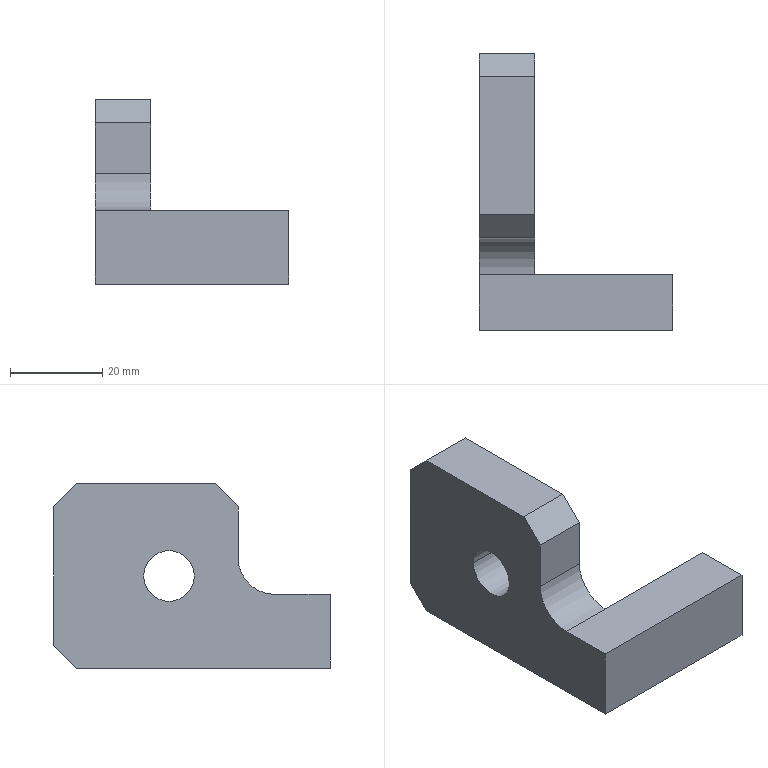Part | STEP file | 012-6-07-010 | 1 solid | 16 faces | box 42 x 60 x 40 mm | volume 27374 mm3 | plane 13 | cylinder 3 | commonest cylinder face diameters 11 x2 16 x1
STEP:
#1=CARTESIAN_POINT('',(0.,0.,0.));
#2=DIRECTION('',(0.,0.,1.));
#3=DIRECTION('',(1.,0.,0.));
#4=AXIS2_PLACEMENT_3D('',#1,#2,#3);
#5=CARTESIAN_POINT('',(0.,40.5,20.));
#6=VERTEX_POINT('',#5);
#7=CARTESIAN_POINT('',(12.,40.5,20.));
#8=VERTEX_POINT('',#7);
#9=CARTESIAN_POINT('',(-13.,40.5,20.));
#10=DIRECTION('',(1.,0.,0.));
#11=VECTOR('',#10,1.);
#12=LINE('',#9,#11);
#13=CARTESIAN_POINT('',(-13.,35.,20.));
#14=DIRECTION('',(1.,0.,0.));
#15=DIRECTION('',(0.,1.,0.));
#16=AXIS2_PLACEMENT_3D('',#13,#14,#15);
#17=CYLINDRICAL_SURFACE('',#16,5.5);
#18=CARTESIAN_POINT('',(6.283,0.));
#19=DIRECTION('',(0.,1.));
#20=VECTOR('',#19,1.);
#21=LINE('',#18,#20);
#22=(GEOMETRIC_REPRESENTATION_CONTEXT(2)PARAMETRIC_REPRESENTATION_CONTEXT()REPRESENTATION_CONTEXT('',''));
#23=DEFINITIONAL_REPRESENTATION('',(#21),#22);
#24=PCURVE('',#17,#23);
#25=CARTESIAN_POINT('',(-13.,35.,20.));
#26=DIRECTION('',(1.,0.,0.));
#27=DIRECTION('',(0.,1.,0.));
#28=AXIS2_PLACEMENT_3D('',#25,#26,#27);
#29=CYLINDRICAL_SURFACE('',#28,5.5);
#30=CARTESIAN_POINT('',(0.,0.));
#31=DIRECTION('',(0.,1.));
#32=VECTOR('',#31,1.);
#33=LINE('',#30,#32);
#34=(GEOMETRIC_REPRESENTATION_CONTEXT(2)PARAMETRIC_REPRESENTATION_CONTEXT()REPRESENTATION_CONTEXT('',''));
#35=DEFINITIONAL_REPRESENTATION('',(#33),#34);
#36=PCURVE('',#29,#35);
#37=SURFACE_CURVE('',#12,(#24,#36),.PCURVE_S1.);
#38=EDGE_CURVE('',#6,#8,#37,.T.);
#39=ORIENTED_EDGE('',*,*,#38,.T.);
#40=CARTESIAN_POINT('',(12.,29.5,20.));
#41=VERTEX_POINT('',#40);
#42=CARTESIAN_POINT('',(12.,35.,20.));
#43=DIRECTION('',(1.,0.,0.));
#44=DIRECTION('',(0.,1.,0.));
#45=AXIS2_PLACEMENT_3D('',#42,#43,#44);
#46=CIRCLE('',#45,5.5);
#47=CARTESIAN_POINT('',(0.,25.));
#48=DIRECTION('',(1.,0.));
#49=VECTOR('',#48,1.);
#50=LINE('',#47,#49);
#51=(GEOMETRIC_REPRESENTATION_CONTEXT(2)PARAMETRIC_REPRESENTATION_CONTEXT()REPRESENTATION_CONTEXT('',''));
#52=DEFINITIONAL_REPRESENTATION('',(#50),#51);
#53=PCURVE('',#17,#52);
#54=CARTESIAN_POINT('',(12.,60.,40.));
#55=DIRECTION('',(-1.,0.,0.));
#56=DIRECTION('',(0.,-1.,0.));
#57=AXIS2_PLACEMENT_3D('',#54,#55,#56);
#58=PLANE('',#57);
#59=CARTESIAN_POINT('',(19.5,-20.));
#60=CARTESIAN_POINT('',(19.5,-10.474));
#61=CARTESIAN_POINT('',(27.75,-15.237));
#62=CARTESIAN_POINT('',(36.,-20.));
#63=CARTESIAN_POINT('',(27.75,-24.763));
#64=CARTESIAN_POINT('',(19.5,-29.526));
#65=CARTESIAN_POINT('',(19.5,-20.));
#66=(BOUNDED_CURVE()B_SPLINE_CURVE(2,(#59,#60,#61,#62,#63,#64,#65),.UNSPECIFIED.,.T.,.F.)B_SPLINE_CURVE_WITH_KNOTS((1,2,2,2,2,1),(-2.094,0.,2.094,4.189,6.283,8.378),.UNSPECIFIED.)CURVE()GEOMETRIC_REPRESENTATION_ITEM()RATIONAL_B_SPLINE_CURVE((1.,0.5,1.,0.5,1.,0.5,1.))REPRESENTATION_ITEM(''));
#67=(GEOMETRIC_REPRESENTATION_CONTEXT(2)PARAMETRIC_REPRESENTATION_CONTEXT()REPRESENTATION_CONTEXT('',''));
#68=DEFINITIONAL_REPRESENTATION('',(#66),#67);
#69=PCURVE('',#58,#68);
#70=SURFACE_CURVE('',#46,(#53,#69),.PCURVE_S1.);
#71=EDGE_CURVE('',#41,#8,#70,.T.);
#72=ORIENTED_EDGE('',*,*,#71,.F.);
#73=CARTESIAN_POINT('',(0.,29.5,20.));
#74=VERTEX_POINT('',#73);
#75=CARTESIAN_POINT('',(-13.,29.5,20.));
#76=DIRECTION('',(1.,0.,0.));
#77=VECTOR('',#76,1.);
#78=LINE('',#75,#77);
#79=CARTESIAN_POINT('',(3.142,0.));
#80=DIRECTION('',(0.,1.));
#81=VECTOR('',#80,1.);
#82=LINE('',#79,#81);
#83=(GEOMETRIC_REPRESENTATION_CONTEXT(2)PARAMETRIC_REPRESENTATION_CONTEXT()REPRESENTATION_CONTEXT('',''));
#84=DEFINITIONAL_REPRESENTATION('',(#82),#83);
#85=PCURVE('',#17,#84);
#86=CARTESIAN_POINT('',(3.142,0.));
#87=DIRECTION('',(0.,1.));
#88=VECTOR('',#87,1.);
#89=LINE('',#86,#88);
#90=(GEOMETRIC_REPRESENTATION_CONTEXT(2)PARAMETRIC_REPRESENTATION_CONTEXT()REPRESENTATION_CONTEXT('',''));
#91=DEFINITIONAL_REPRESENTATION('',(#89),#90);
#92=PCURVE('',#29,#91);
#93=SURFACE_CURVE('',#78,(#85,#92),.PCURVE_S1.);
#94=EDGE_CURVE('',#74,#41,#93,.T.);
#95=ORIENTED_EDGE('',*,*,#94,.F.);
#96=CARTESIAN_POINT('',(0.,35.,20.));
#97=DIRECTION('',(1.,0.,0.));
#98=DIRECTION('',(0.,0.,-1.));
#99=AXIS2_PLACEMENT_3D('',#96,#97,#98);
#100=CIRCLE('',#99,5.5);
#101=CARTESIAN_POINT('',(-1.571,13.));
#102=DIRECTION('',(1.,0.));
#103=VECTOR('',#102,1.);
#104=LINE('',#101,#103);
#105=(GEOMETRIC_REPRESENTATION_CONTEXT(2)PARAMETRIC_REPRESENTATION_CONTEXT()REPRESENTATION_CONTEXT('',''));
#106=DEFINITIONAL_REPRESENTATION('',(#104),#105);
#107=PCURVE('',#17,#106);
#108=CARTESIAN_POINT('',(0.,0.,40.));
#109=DIRECTION('',(1.,0.,0.));
#110=DIRECTION('',(0.,0.,-1.));
#111=AXIS2_PLACEMENT_3D('',#108,#109,#110);
#112=PLANE('',#111);
#113=CARTESIAN_POINT('',(20.,35.));
#114=DIRECTION('',(1.,0.));
#115=AXIS2_PLACEMENT_2D('',#113,#114);
#116=CIRCLE('',#115,5.5);
#117=(GEOMETRIC_REPRESENTATION_CONTEXT(2)PARAMETRIC_REPRESENTATION_CONTEXT()REPRESENTATION_CONTEXT('',''));
#118=DEFINITIONAL_REPRESENTATION('',(#116),#117);
#119=PCURVE('',#112,#118);
#120=SURFACE_CURVE('',#100,(#107,#119),.PCURVE_S1.);
#121=EDGE_CURVE('',#74,#6,#120,.T.);
#122=ORIENTED_EDGE('',*,*,#121,.T.);
#123=EDGE_LOOP('',(#39,#72,#95,#122));
#124=FACE_BOUND('',#123,.F.);
#125=ADVANCED_FACE('',(#124),#17,.F.);
#126=CARTESIAN_POINT('',(0.,0.,16.));
#127=VERTEX_POINT('',#126);
#128=CARTESIAN_POINT('',(42.,0.,16.));
#129=VERTEX_POINT('',#128);
#130=CARTESIAN_POINT('',(42.,0.,16.));
#131=DIRECTION('',(1.,0.,0.));
#132=VECTOR('',#131,1.);
#133=LINE('',#130,#132);
#134=CARTESIAN_POINT('',(0.,0.,40.));
#135=DIRECTION('',(0.,1.,0.));
#136=DIRECTION('',(0.,0.,1.));
#137=AXIS2_PLACEMENT_3D('',#134,#135,#136);
#138=PLANE('',#137);
#139=CARTESIAN_POINT('',(-24.,42.));
#140=DIRECTION('',(0.,1.));
#141=VECTOR('',#140,1.);
#142=LINE('',#139,#141);
#143=(GEOMETRIC_REPRESENTATION_CONTEXT(2)PARAMETRIC_REPRESENTATION_CONTEXT()REPRESENTATION_CONTEXT('',''));
#144=DEFINITIONAL_REPRESENTATION('',(#142),#143);
#145=PCURVE('',#138,#144);
#146=CARTESIAN_POINT('',(42.,20.,16.));
#147=DIRECTION('',(0.,0.,1.));
#148=DIRECTION('',(1.,0.,0.));
#149=AXIS2_PLACEMENT_3D('',#146,#147,#148);
#150=PLANE('',#149);
#151=CARTESIAN_POINT('',(0.,-20.));
#152=DIRECTION('',(1.,0.));
#153=VECTOR('',#152,1.);
#154=LINE('',#151,#153);
#155=(GEOMETRIC_REPRESENTATION_CONTEXT(2)PARAMETRIC_REPRESENTATION_CONTEXT()REPRESENTATION_CONTEXT('',''));
#156=DEFINITIONAL_REPRESENTATION('',(#154),#155);
#157=PCURVE('',#150,#156);
#158=SURFACE_CURVE('',#133,(#145,#157),.PCURVE_S1.);
#159=EDGE_CURVE('',#127,#129,#158,.T.);
#160=ORIENTED_EDGE('',*,*,#159,.F.);
#161=CARTESIAN_POINT('',(0.,0.,0.));
#162=VERTEX_POINT('',#161);
#163=CARTESIAN_POINT('',(0.,0.,40.));
#164=DIRECTION('',(0.,0.,-1.));
#165=VECTOR('',#164,1.);
#166=LINE('',#163,#165);
#167=CARTESIAN_POINT('',(0.,0.));
#168=DIRECTION('',(-1.,0.));
#169=VECTOR('',#168,1.);
#170=LINE('',#167,#169);
#171=(GEOMETRIC_REPRESENTATION_CONTEXT(2)PARAMETRIC_REPRESENTATION_CONTEXT()REPRESENTATION_CONTEXT('',''));
#172=DEFINITIONAL_REPRESENTATION('',(#170),#171);
#173=PCURVE('',#138,#172);
#174=CARTESIAN_POINT('',(0.,0.));
#175=DIRECTION('',(1.,0.));
#176=VECTOR('',#175,1.);
#177=LINE('',#174,#176);
#178=(GEOMETRIC_REPRESENTATION_CONTEXT(2)PARAMETRIC_REPRESENTATION_CONTEXT()REPRESENTATION_CONTEXT('',''));
#179=DEFINITIONAL_REPRESENTATION('',(#177),#178);
#180=PCURVE('',#112,#179);
#181=SURFACE_CURVE('',#166,(#173,#180),.PCURVE_S1.);
#182=EDGE_CURVE('',#127,#162,#181,.T.);
#183=ORIENTED_EDGE('',*,*,#182,.T.);
#184=CARTESIAN_POINT('',(42.,0.,0.));
#185=VERTEX_POINT('',#184);
#186=CARTESIAN_POINT('',(0.,0.,0.));
#187=DIRECTION('',(1.,0.,0.));
#188=VECTOR('',#187,1.);
#189=LINE('',#186,#188);
#190=CARTESIAN_POINT('',(-40.,0.));
#191=DIRECTION('',(0.,1.));
#192=VECTOR('',#191,1.);
#193=LINE('',#190,#192);
#194=(GEOMETRIC_REPRESENTATION_CONTEXT(2)PARAMETRIC_REPRESENTATION_CONTEXT()REPRESENTATION_CONTEXT('',''));
#195=DEFINITIONAL_REPRESENTATION('',(#193),#194);
#196=PCURVE('',#138,#195);
#197=CARTESIAN_POINT('',(0.,60.,0.));
#198=DIRECTION('',(0.,0.,-1.));
#199=DIRECTION('',(-1.,0.,0.));
#200=AXIS2_PLACEMENT_3D('',#197,#198,#199);
#201=PLANE('',#200);
#202=CARTESIAN_POINT('',(0.,-60.));
#203=DIRECTION('',(-1.,0.));
#204=VECTOR('',#203,1.);
#205=LINE('',#202,#204);
#206=(GEOMETRIC_REPRESENTATION_CONTEXT(2)PARAMETRIC_REPRESENTATION_CONTEXT()REPRESENTATION_CONTEXT('',''));
#207=DEFINITIONAL_REPRESENTATION('',(#205),#206);
#208=PCURVE('',#201,#207);
#209=SURFACE_CURVE('',#189,(#196,#208),.PCURVE_S1.);
#210=EDGE_CURVE('',#162,#185,#209,.T.);
#211=ORIENTED_EDGE('',*,*,#210,.T.);
#212=CARTESIAN_POINT('',(42.,0.,40.));
#213=DIRECTION('',(0.,0.,-1.));
#214=VECTOR('',#213,1.);
#215=LINE('',#212,#214);
#216=CARTESIAN_POINT('',(0.,42.));
#217=DIRECTION('',(-1.,0.));
#218=VECTOR('',#217,1.);
#219=LINE('',#216,#218);
#220=(GEOMETRIC_REPRESENTATION_CONTEXT(2)PARAMETRIC_REPRESENTATION_CONTEXT()REPRESENTATION_CONTEXT('',''));
#221=DEFINITIONAL_REPRESENTATION('',(#219),#220);
#222=PCURVE('',#138,#221);
#223=CARTESIAN_POINT('',(42.,0.,40.));
#224=DIRECTION('',(-1.,0.,0.));
#225=DIRECTION('',(0.,0.,1.));
#226=AXIS2_PLACEMENT_3D('',#223,#224,#225);
#227=PLANE('',#226);
#228=CARTESIAN_POINT('',(0.,0.));
#229=DIRECTION('',(-1.,0.));
#230=VECTOR('',#229,1.);
#231=LINE('',#228,#230);
#232=(GEOMETRIC_REPRESENTATION_CONTEXT(2)PARAMETRIC_REPRESENTATION_CONTEXT()REPRESENTATION_CONTEXT('',''));
#233=DEFINITIONAL_REPRESENTATION('',(#231),#232);
#234=PCURVE('',#227,#233);
#235=SURFACE_CURVE('',#215,(#222,#234),.PCURVE_S1.);
#236=EDGE_CURVE('',#129,#185,#235,.T.);
#237=ORIENTED_EDGE('',*,*,#236,.F.);
#238=EDGE_LOOP('',(#160,#183,#211,#237));
#239=FACE_BOUND('',#238,.T.);
#240=ADVANCED_FACE('',(#239),#138,.F.);
#241=CARTESIAN_POINT('',(42.,12.,16.));
#242=VERTEX_POINT('',#241);
#243=CARTESIAN_POINT('',(42.,0.,16.));
#244=DIRECTION('',(0.,1.,0.));
#245=VECTOR('',#244,1.);
#246=LINE('',#243,#245);
#247=CARTESIAN_POINT('',(-24.,0.));
#248=DIRECTION('',(0.,1.));
#249=VECTOR('',#248,1.);
#250=LINE('',#247,#249);
#251=(GEOMETRIC_REPRESENTATION_CONTEXT(2)PARAMETRIC_REPRESENTATION_CONTEXT()REPRESENTATION_CONTEXT('',''));
#252=DEFINITIONAL_REPRESENTATION('',(#250),#251);
#253=PCURVE('',#227,#252);
#254=CARTESIAN_POINT('',(0.,-20.));
#255=DIRECTION('',(0.,1.));
#256=VECTOR('',#255,1.);
#257=LINE('',#254,#256);
#258=(GEOMETRIC_REPRESENTATION_CONTEXT(2)PARAMETRIC_REPRESENTATION_CONTEXT()REPRESENTATION_CONTEXT('',''));
#259=DEFINITIONAL_REPRESENTATION('',(#257),#258);
#260=PCURVE('',#150,#259);
#261=SURFACE_CURVE('',#246,(#253,#260),.PCURVE_S1.);
#262=EDGE_CURVE('',#129,#242,#261,.T.);
#263=ORIENTED_EDGE('',*,*,#262,.F.);
#264=ORIENTED_EDGE('',*,*,#236,.T.);
#265=CARTESIAN_POINT('',(42.,12.,0.));
#266=VERTEX_POINT('',#265);
#267=CARTESIAN_POINT('',(42.,0.,0.));
#268=DIRECTION('',(0.,1.,0.));
#269=VECTOR('',#268,1.);
#270=LINE('',#267,#269);
#271=CARTESIAN_POINT('',(-40.,0.));
#272=DIRECTION('',(0.,1.));
#273=VECTOR('',#272,1.);
#274=LINE('',#271,#273);
#275=(GEOMETRIC_REPRESENTATION_CONTEXT(2)PARAMETRIC_REPRESENTATION_CONTEXT()REPRESENTATION_CONTEXT('',''));
#276=DEFINITIONAL_REPRESENTATION('',(#274),#275);
#277=PCURVE('',#227,#276);
#278=CARTESIAN_POINT('',(-42.,-60.));
#279=DIRECTION('',(0.,1.));
#280=VECTOR('',#279,1.);
#281=LINE('',#278,#280);
#282=(GEOMETRIC_REPRESENTATION_CONTEXT(2)PARAMETRIC_REPRESENTATION_CONTEXT()REPRESENTATION_CONTEXT('',''));
#283=DEFINITIONAL_REPRESENTATION('',(#281),#282);
#284=PCURVE('',#201,#283);
#285=SURFACE_CURVE('',#270,(#277,#284),.PCURVE_S1.);
#286=EDGE_CURVE('',#185,#266,#285,.T.);
#287=ORIENTED_EDGE('',*,*,#286,.T.);
#288=CARTESIAN_POINT('',(42.,12.,40.));
#289=DIRECTION('',(0.,0.,-1.));
#290=VECTOR('',#289,1.);
#291=LINE('',#288,#290);
#292=CARTESIAN_POINT('',(0.,12.));
#293=DIRECTION('',(-1.,0.));
#294=VECTOR('',#293,1.);
#295=LINE('',#292,#294);
#296=(GEOMETRIC_REPRESENTATION_CONTEXT(2)PARAMETRIC_REPRESENTATION_CONTEXT()REPRESENTATION_CONTEXT('',''));
#297=DEFINITIONAL_REPRESENTATION('',(#295),#296);
#298=PCURVE('',#227,#297);
#299=CARTESIAN_POINT('',(12.,12.,40.));
#300=DIRECTION('',(0.,-1.,0.));
#301=DIRECTION('',(0.,0.,-1.));
#302=AXIS2_PLACEMENT_3D('',#299,#300,#301);
#303=PLANE('',#302);
#304=CARTESIAN_POINT('',(0.,30.));
#305=DIRECTION('',(1.,0.));
#306=VECTOR('',#305,1.);
#307=LINE('',#304,#306);
#308=(GEOMETRIC_REPRESENTATION_CONTEXT(2)PARAMETRIC_REPRESENTATION_CONTEXT()REPRESENTATION_CONTEXT('',''));
#309=DEFINITIONAL_REPRESENTATION('',(#307),#308);
#310=PCURVE('',#303,#309);
#311=SURFACE_CURVE('',#291,(#298,#310),.PCURVE_S1.);
#312=EDGE_CURVE('',#242,#266,#311,.T.);
#313=ORIENTED_EDGE('',*,*,#312,.F.);
#314=EDGE_LOOP('',(#263,#264,#287,#313));
#315=FACE_BOUND('',#314,.T.);
#316=ADVANCED_FACE('',(#315),#227,.F.);
#317=CARTESIAN_POINT('',(12.,12.,16.));
#318=VERTEX_POINT('',#317);
#319=CARTESIAN_POINT('',(12.,12.,16.));
#320=DIRECTION('',(-1.,0.,0.));
#321=VECTOR('',#320,1.);
#322=LINE('',#319,#321);
#323=CARTESIAN_POINT('',(24.,0.));
#324=DIRECTION('',(0.,-1.));
#325=VECTOR('',#324,1.);
#326=LINE('',#323,#325);
#327=(GEOMETRIC_REPRESENTATION_CONTEXT(2)PARAMETRIC_REPRESENTATION_CONTEXT()REPRESENTATION_CONTEXT('',''));
#328=DEFINITIONAL_REPRESENTATION('',(#326),#327);
#329=PCURVE('',#303,#328);
#330=CARTESIAN_POINT('',(-30.,-8.));
#331=DIRECTION('',(-1.,0.));
#332=VECTOR('',#331,1.);
#333=LINE('',#330,#332);
#334=(GEOMETRIC_REPRESENTATION_CONTEXT(2)PARAMETRIC_REPRESENTATION_CONTEXT()REPRESENTATION_CONTEXT('',''));
#335=DEFINITIONAL_REPRESENTATION('',(#333),#334);
#336=PCURVE('',#150,#335);
#337=SURFACE_CURVE('',#322,(#329,#336),.PCURVE_S1.);
#338=EDGE_CURVE('',#242,#318,#337,.T.);
#339=ORIENTED_EDGE('',*,*,#338,.F.);
#340=ORIENTED_EDGE('',*,*,#312,.T.);
#341=CARTESIAN_POINT('',(12.,12.,0.));
#342=VERTEX_POINT('',#341);
#343=CARTESIAN_POINT('',(12.,12.,0.));
#344=DIRECTION('',(-1.,0.,0.));
#345=VECTOR('',#344,1.);
#346=LINE('',#343,#345);
#347=CARTESIAN_POINT('',(40.,0.));
#348=DIRECTION('',(0.,-1.));
#349=VECTOR('',#348,1.);
#350=LINE('',#347,#349);
#351=(GEOMETRIC_REPRESENTATION_CONTEXT(2)PARAMETRIC_REPRESENTATION_CONTEXT()REPRESENTATION_CONTEXT('',''));
#352=DEFINITIONAL_REPRESENTATION('',(#350),#351);
#353=PCURVE('',#303,#352);
#354=CARTESIAN_POINT('',(-12.,-48.));
#355=DIRECTION('',(1.,0.));
#356=VECTOR('',#355,1.);
#357=LINE('',#354,#356);
#358=(GEOMETRIC_REPRESENTATION_CONTEXT(2)PARAMETRIC_REPRESENTATION_CONTEXT()REPRESENTATION_CONTEXT('',''));
#359=DEFINITIONAL_REPRESENTATION('',(#357),#358);
#360=PCURVE('',#201,#359);
#361=SURFACE_CURVE('',#346,(#353,#360),.PCURVE_S1.);
#362=EDGE_CURVE('',#266,#342,#361,.T.);
#363=ORIENTED_EDGE('',*,*,#362,.T.);
#364=CARTESIAN_POINT('',(12.,12.,40.));
#365=DIRECTION('',(0.,0.,-1.));
#366=VECTOR('',#365,1.);
#367=LINE('',#364,#366);
#368=CARTESIAN_POINT('',(0.,0.));
#369=DIRECTION('',(1.,0.));
#370=VECTOR('',#369,1.);
#371=LINE('',#368,#370);
#372=(GEOMETRIC_REPRESENTATION_CONTEXT(2)PARAMETRIC_REPRESENTATION_CONTEXT()REPRESENTATION_CONTEXT('',''));
#373=DEFINITIONAL_REPRESENTATION('',(#371),#372);
#374=PCURVE('',#303,#373);
#375=CARTESIAN_POINT('',(48.,0.));
#376=DIRECTION('',(0.,-1.));
#377=VECTOR('',#376,1.);
#378=LINE('',#375,#377);
#379=(GEOMETRIC_REPRESENTATION_CONTEXT(2)PARAMETRIC_REPRESENTATION_CONTEXT()REPRESENTATION_CONTEXT('',''));
#380=DEFINITIONAL_REPRESENTATION('',(#378),#379);
#381=PCURVE('',#58,#380);
#382=SURFACE_CURVE('',#367,(#374,#381),.PCURVE_S1.);
#383=EDGE_CURVE('',#318,#342,#382,.T.);
#384=ORIENTED_EDGE('',*,*,#383,.F.);
#385=EDGE_LOOP('',(#339,#340,#363,#384));
#386=FACE_BOUND('',#385,.T.);
#387=ADVANCED_FACE('',(#386),#303,.F.);
#388=CARTESIAN_POINT('',(0.,35.,20.));
#389=DIRECTION('',(1.,0.,0.));
#390=DIRECTION('',(0.,0.,-1.));
#391=AXIS2_PLACEMENT_3D('',#388,#389,#390);
#392=CIRCLE('',#391,5.5);
#393=CARTESIAN_POINT('',(20.,35.));
#394=DIRECTION('',(1.,0.));
#395=AXIS2_PLACEMENT_2D('',#393,#394);
#396=CIRCLE('',#395,5.5);
#397=(GEOMETRIC_REPRESENTATION_CONTEXT(2)PARAMETRIC_REPRESENTATION_CONTEXT()REPRESENTATION_CONTEXT('',''));
#398=DEFINITIONAL_REPRESENTATION('',(#396),#397);
#399=PCURVE('',#112,#398);
#400=CARTESIAN_POINT('',(-1.571,13.));
#401=DIRECTION('',(1.,0.));
#402=VECTOR('',#401,1.);
#403=LINE('',#400,#402);
#404=(GEOMETRIC_REPRESENTATION_CONTEXT(2)PARAMETRIC_REPRESENTATION_CONTEXT()REPRESENTATION_CONTEXT('',''));
#405=DEFINITIONAL_REPRESENTATION('',(#403),#404);
#406=PCURVE('',#29,#405);
#407=SURFACE_CURVE('',#392,(#399,#406),.PCURVE_S1.);
#408=EDGE_CURVE('',#6,#74,#407,.T.);
#409=ORIENTED_EDGE('',*,*,#408,.T.);
#410=ORIENTED_EDGE('',*,*,#121,.T.);
#411=EDGE_LOOP('',(#409,#410));
#412=FACE_BOUND('',#411,.T.);
#413=CARTESIAN_POINT('',(0.,20.,24.));
#414=VERTEX_POINT('',#413);
#415=CARTESIAN_POINT('',(0.,20.,35.));
#416=VERTEX_POINT('',#415);
#417=CARTESIAN_POINT('',(0.,20.,16.));
#418=DIRECTION('',(0.,0.,1.));
#419=VECTOR('',#418,1.);
#420=LINE('',#417,#419);
#421=CARTESIAN_POINT('',(24.,20.));
#422=DIRECTION('',(-1.,0.));
#423=VECTOR('',#422,1.);
#424=LINE('',#421,#423);
#425=(GEOMETRIC_REPRESENTATION_CONTEXT(2)PARAMETRIC_REPRESENTATION_CONTEXT()REPRESENTATION_CONTEXT('',''));
#426=DEFINITIONAL_REPRESENTATION('',(#424),#425);
#427=PCURVE('',#112,#426);
#428=CARTESIAN_POINT('',(42.,20.,16.));
#429=DIRECTION('',(0.,1.,0.));
#430=DIRECTION('',(-1.,0.,0.));
#431=AXIS2_PLACEMENT_3D('',#428,#429,#430);
#432=PLANE('',#431);
#433=CARTESIAN_POINT('',(42.,0.));
#434=DIRECTION('',(0.,1.));
#435=VECTOR('',#434,1.);
#436=LINE('',#433,#435);
#437=(GEOMETRIC_REPRESENTATION_CONTEXT(2)PARAMETRIC_REPRESENTATION_CONTEXT()REPRESENTATION_CONTEXT('',''));
#438=DEFINITIONAL_REPRESENTATION('',(#436),#437);
#439=PCURVE('',#432,#438);
#440=SURFACE_CURVE('',#420,(#427,#439),.PCURVE_S1.);
#441=EDGE_CURVE('',#414,#416,#440,.T.);
#442=ORIENTED_EDGE('',*,*,#441,.T.);
#443=CARTESIAN_POINT('',(0.,25.,40.));
#444=VERTEX_POINT('',#443);
#445=CARTESIAN_POINT('',(0.,25.,40.));
#446=DIRECTION('',(0.,0.7071,0.7071));
#447=VECTOR('',#446,1.);
#448=LINE('',#445,#447);
#449=CARTESIAN_POINT('',(0.,25.));
#450=DIRECTION('',(-0.7071,0.7071));
#451=VECTOR('',#450,1.);
#452=LINE('',#449,#451);
#453=(GEOMETRIC_REPRESENTATION_CONTEXT(2)PARAMETRIC_REPRESENTATION_CONTEXT()REPRESENTATION_CONTEXT('',''));
#454=DEFINITIONAL_REPRESENTATION('',(#452),#453);
#455=PCURVE('',#112,#454);
#456=CARTESIAN_POINT('',(0.,25.,40.));
#457=DIRECTION('',(0.,0.7071,-0.7071));
#458=DIRECTION('',(0.,0.7071,0.7071));
#459=AXIS2_PLACEMENT_3D('',#456,#457,#458);
#460=PLANE('',#459);
#461=CARTESIAN_POINT('',(0.,0.));
#462=DIRECTION('',(1.,0.));
#463=VECTOR('',#462,1.);
#464=LINE('',#461,#463);
#465=(GEOMETRIC_REPRESENTATION_CONTEXT(2)PARAMETRIC_REPRESENTATION_CONTEXT()REPRESENTATION_CONTEXT('',''));
#466=DEFINITIONAL_REPRESENTATION('',(#464),#465);
#467=PCURVE('',#460,#466);
#468=SURFACE_CURVE('',#448,(#455,#467),.PCURVE_S1.);
#469=EDGE_CURVE('',#416,#444,#468,.T.);
#470=ORIENTED_EDGE('',*,*,#469,.T.);
#471=CARTESIAN_POINT('',(0.,55.,40.));
#472=VERTEX_POINT('',#471);
#473=CARTESIAN_POINT('',(0.,0.,40.));
#474=DIRECTION('',(0.,-1.,0.));
#475=VECTOR('',#474,1.);
#476=LINE('',#473,#475);
#477=CARTESIAN_POINT('',(0.,0.));
#478=DIRECTION('',(0.,-1.));
#479=VECTOR('',#478,1.);
#480=LINE('',#477,#479);
#481=(GEOMETRIC_REPRESENTATION_CONTEXT(2)PARAMETRIC_REPRESENTATION_CONTEXT()REPRESENTATION_CONTEXT('',''));
#482=DEFINITIONAL_REPRESENTATION('',(#480),#481);
#483=PCURVE('',#112,#482);
#484=CARTESIAN_POINT('',(0.,60.,40.));
#485=DIRECTION('',(0.,0.,-1.));
#486=DIRECTION('',(-1.,0.,0.));
#487=AXIS2_PLACEMENT_3D('',#484,#485,#486);
#488=PLANE('',#487);
#489=CARTESIAN_POINT('',(0.,-60.));
#490=DIRECTION('',(0.,-1.));
#491=VECTOR('',#490,1.);
#492=LINE('',#489,#491);
#493=(GEOMETRIC_REPRESENTATION_CONTEXT(2)PARAMETRIC_REPRESENTATION_CONTEXT()REPRESENTATION_CONTEXT('',''));
#494=DEFINITIONAL_REPRESENTATION('',(#492),#493);
#495=PCURVE('',#488,#494);
#496=SURFACE_CURVE('',#476,(#483,#495),.PCURVE_S1.);
#497=EDGE_CURVE('',#472,#444,#496,.T.);
#498=ORIENTED_EDGE('',*,*,#497,.F.);
#499=CARTESIAN_POINT('',(0.,60.,35.));
#500=VERTEX_POINT('',#499);
#501=CARTESIAN_POINT('',(0.,55.,40.));
#502=DIRECTION('',(0.,0.7071,-0.7071));
#503=VECTOR('',#502,1.);
#504=LINE('',#501,#503);
#505=CARTESIAN_POINT('',(0.,55.));
#506=DIRECTION('',(0.7071,0.7071));
#507=VECTOR('',#506,1.);
#508=LINE('',#505,#507);
#509=(GEOMETRIC_REPRESENTATION_CONTEXT(2)PARAMETRIC_REPRESENTATION_CONTEXT()REPRESENTATION_CONTEXT('',''));
#510=DEFINITIONAL_REPRESENTATION('',(#508),#509);
#511=PCURVE('',#112,#510);
#512=CARTESIAN_POINT('',(0.,55.,40.));
#513=DIRECTION('',(0.,-0.7071,-0.7071));
#514=DIRECTION('',(0.,0.7071,-0.7071));
#515=AXIS2_PLACEMENT_3D('',#512,#513,#514);
#516=PLANE('',#515);
#517=CARTESIAN_POINT('',(0.,0.));
#518=DIRECTION('',(1.,0.));
#519=VECTOR('',#518,1.);
#520=LINE('',#517,#519);
#521=(GEOMETRIC_REPRESENTATION_CONTEXT(2)PARAMETRIC_REPRESENTATION_CONTEXT()REPRESENTATION_CONTEXT('',''));
#522=DEFINITIONAL_REPRESENTATION('',(#520),#521);
#523=PCURVE('',#516,#522);
#524=SURFACE_CURVE('',#504,(#511,#523),.PCURVE_S1.);
#525=EDGE_CURVE('',#472,#500,#524,.T.);
#526=ORIENTED_EDGE('',*,*,#525,.T.);
#527=CARTESIAN_POINT('',(0.,60.,5.));
#528=VERTEX_POINT('',#527);
#529=CARTESIAN_POINT('',(0.,60.,40.));
#530=DIRECTION('',(0.,0.,-1.));
#531=VECTOR('',#530,1.);
#532=LINE('',#529,#531);
#533=CARTESIAN_POINT('',(0.,60.));
#534=DIRECTION('',(1.,0.));
#535=VECTOR('',#534,1.);
#536=LINE('',#533,#535);
#537=(GEOMETRIC_REPRESENTATION_CONTEXT(2)PARAMETRIC_REPRESENTATION_CONTEXT()REPRESENTATION_CONTEXT('',''));
#538=DEFINITIONAL_REPRESENTATION('',(#536),#537);
#539=PCURVE('',#112,#538);
#540=CARTESIAN_POINT('',(0.,60.,40.));
#541=DIRECTION('',(0.,-1.,0.));
#542=DIRECTION('',(0.,0.,-1.));
#543=AXIS2_PLACEMENT_3D('',#540,#541,#542);
#544=PLANE('',#543);
#545=CARTESIAN_POINT('',(0.,0.));
#546=DIRECTION('',(1.,0.));
#547=VECTOR('',#546,1.);
#548=LINE('',#545,#547);
#549=(GEOMETRIC_REPRESENTATION_CONTEXT(2)PARAMETRIC_REPRESENTATION_CONTEXT()REPRESENTATION_CONTEXT('',''));
#550=DEFINITIONAL_REPRESENTATION('',(#548),#549);
#551=PCURVE('',#544,#550);
#552=SURFACE_CURVE('',#532,(#539,#551),.PCURVE_S1.);
#553=EDGE_CURVE('',#500,#528,#552,.T.);
#554=ORIENTED_EDGE('',*,*,#553,.T.);
#555=CARTESIAN_POINT('',(0.,55.,0.));
#556=VERTEX_POINT('',#555);
#557=CARTESIAN_POINT('',(0.,60.,5.));
#558=DIRECTION('',(0.,-0.7071,-0.7071));
#559=VECTOR('',#558,1.);
#560=LINE('',#557,#559);
#561=CARTESIAN_POINT('',(35.,60.));
#562=DIRECTION('',(0.7071,-0.7071));
#563=VECTOR('',#562,1.);
#564=LINE('',#561,#563);
#565=(GEOMETRIC_REPRESENTATION_CONTEXT(2)PARAMETRIC_REPRESENTATION_CONTEXT()REPRESENTATION_CONTEXT('',''));
#566=DEFINITIONAL_REPRESENTATION('',(#564),#565);
#567=PCURVE('',#112,#566);
#568=CARTESIAN_POINT('',(0.,60.,5.));
#569=DIRECTION('',(0.,0.7071,-0.7071));
#570=DIRECTION('',(0.,0.7071,0.7071));
#571=AXIS2_PLACEMENT_3D('',#568,#569,#570);
#572=PLANE('',#571);
#573=CARTESIAN_POINT('',(0.,0.));
#574=DIRECTION('',(-1.,0.));
#575=VECTOR('',#574,1.);
#576=LINE('',#573,#575);
#577=(GEOMETRIC_REPRESENTATION_CONTEXT(2)PARAMETRIC_REPRESENTATION_CONTEXT()REPRESENTATION_CONTEXT('',''));
#578=DEFINITIONAL_REPRESENTATION('',(#576),#577);
#579=PCURVE('',#572,#578);
#580=SURFACE_CURVE('',#560,(#567,#579),.PCURVE_S1.);
#581=EDGE_CURVE('',#528,#556,#580,.T.);
#582=ORIENTED_EDGE('',*,*,#581,.T.);
#583=CARTESIAN_POINT('',(0.,0.,0.));
#584=DIRECTION('',(0.,-1.,0.));
#585=VECTOR('',#584,1.);
#586=LINE('',#583,#585);
#587=CARTESIAN_POINT('',(40.,0.));
#588=DIRECTION('',(0.,-1.));
#589=VECTOR('',#588,1.);
#590=LINE('',#587,#589);
#591=(GEOMETRIC_REPRESENTATION_CONTEXT(2)PARAMETRIC_REPRESENTATION_CONTEXT()REPRESENTATION_CONTEXT('',''));
#592=DEFINITIONAL_REPRESENTATION('',(#590),#591);
#593=PCURVE('',#112,#592);
#594=CARTESIAN_POINT('',(0.,-60.));
#595=DIRECTION('',(0.,-1.));
#596=VECTOR('',#595,1.);
#597=LINE('',#594,#596);
#598=(GEOMETRIC_REPRESENTATION_CONTEXT(2)PARAMETRIC_REPRESENTATION_CONTEXT()REPRESENTATION_CONTEXT('',''));
#599=DEFINITIONAL_REPRESENTATION('',(#597),#598);
#600=PCURVE('',#201,#599);
#601=SURFACE_CURVE('',#586,(#593,#600),.PCURVE_S1.);
#602=EDGE_CURVE('',#556,#162,#601,.T.);
#603=ORIENTED_EDGE('',*,*,#602,.T.);
#604=ORIENTED_EDGE('',*,*,#182,.F.);
#605=CARTESIAN_POINT('',(0.,12.,16.));
#606=VERTEX_POINT('',#605);
#607=CARTESIAN_POINT('',(0.,0.,16.));
#608=DIRECTION('',(0.,-1.,0.));
#609=VECTOR('',#608,1.);
#610=LINE('',#607,#609);
#611=CARTESIAN_POINT('',(24.,0.));
#612=DIRECTION('',(0.,-1.));
#613=VECTOR('',#612,1.);
#614=LINE('',#611,#613);
#615=(GEOMETRIC_REPRESENTATION_CONTEXT(2)PARAMETRIC_REPRESENTATION_CONTEXT()REPRESENTATION_CONTEXT('',''));
#616=DEFINITIONAL_REPRESENTATION('',(#614),#615);
#617=PCURVE('',#112,#616);
#618=CARTESIAN_POINT('',(-42.,-20.));
#619=DIRECTION('',(0.,-1.));
#620=VECTOR('',#619,1.);
#621=LINE('',#618,#620);
#622=(GEOMETRIC_REPRESENTATION_CONTEXT(2)PARAMETRIC_REPRESENTATION_CONTEXT()REPRESENTATION_CONTEXT('',''));
#623=DEFINITIONAL_REPRESENTATION('',(#621),#622);
#624=PCURVE('',#150,#623);
#625=SURFACE_CURVE('',#610,(#617,#624),.PCURVE_S1.);
#626=EDGE_CURVE('',#606,#127,#625,.T.);
#627=ORIENTED_EDGE('',*,*,#626,.F.);
#628=CARTESIAN_POINT('',(0.,12.,24.));
#629=DIRECTION('',(1.,0.,0.));
#630=DIRECTION('',(0.,0.,-1.));
#631=AXIS2_PLACEMENT_3D('',#628,#629,#630);
#632=CIRCLE('',#631,8.);
#633=CARTESIAN_POINT('',(16.,12.));
#634=DIRECTION('',(1.,0.));
#635=AXIS2_PLACEMENT_2D('',#633,#634);
#636=CIRCLE('',#635,8.);
#637=(GEOMETRIC_REPRESENTATION_CONTEXT(2)PARAMETRIC_REPRESENTATION_CONTEXT()REPRESENTATION_CONTEXT('',''));
#638=DEFINITIONAL_REPRESENTATION('',(#636),#637);
#639=PCURVE('',#112,#638);
#640=CARTESIAN_POINT('',(42.,12.,24.));
#641=DIRECTION('',(-1.,0.,0.));
#642=DIRECTION('',(0.,-1.,0.));
#643=AXIS2_PLACEMENT_3D('',#640,#641,#642);
#644=CYLINDRICAL_SURFACE('',#643,8.);
#645=CARTESIAN_POINT('',(4.712,42.));
#646=DIRECTION('',(-1.,0.));
#647=VECTOR('',#646,1.);
#648=LINE('',#645,#647);
#649=(GEOMETRIC_REPRESENTATION_CONTEXT(2)PARAMETRIC_REPRESENTATION_CONTEXT()REPRESENTATION_CONTEXT('',''));
#650=DEFINITIONAL_REPRESENTATION('',(#648),#649);
#651=PCURVE('',#644,#650);
#652=SURFACE_CURVE('',#632,(#639,#651),.PCURVE_S1.);
#653=EDGE_CURVE('',#606,#414,#652,.T.);
#654=ORIENTED_EDGE('',*,*,#653,.T.);
#655=EDGE_LOOP('',(#442,#470,#498,#526,#554,#582,#603,#604,#627,#654));
#656=FACE_BOUND('',#655,.T.);
#657=ADVANCED_FACE('',(#412,#656),#112,.F.);
#658=CARTESIAN_POINT('',(12.,35.,20.));
#659=DIRECTION('',(1.,0.,0.));
#660=DIRECTION('',(0.,1.,0.));
#661=AXIS2_PLACEMENT_3D('',#658,#659,#660);
#662=CIRCLE('',#661,5.5);
#663=CARTESIAN_POINT('',(19.5,-20.));
#664=CARTESIAN_POINT('',(19.5,-10.474));
#665=CARTESIAN_POINT('',(27.75,-15.237));
#666=CARTESIAN_POINT('',(36.,-20.));
#667=CARTESIAN_POINT('',(27.75,-24.763));
#668=CARTESIAN_POINT('',(19.5,-29.526));
#669=CARTESIAN_POINT('',(19.5,-20.));
#670=(BOUNDED_CURVE()B_SPLINE_CURVE(2,(#663,#664,#665,#666,#667,#668,#669),.UNSPECIFIED.,.T.,.F.)B_SPLINE_CURVE_WITH_KNOTS((1,2,2,2,2,1),(-2.094,0.,2.094,4.189,6.283,8.378),.UNSPECIFIED.)CURVE()GEOMETRIC_REPRESENTATION_ITEM()RATIONAL_B_SPLINE_CURVE((1.,0.5,1.,0.5,1.,0.5,1.))REPRESENTATION_ITEM(''));
#671=(GEOMETRIC_REPRESENTATION_CONTEXT(2)PARAMETRIC_REPRESENTATION_CONTEXT()REPRESENTATION_CONTEXT('',''));
#672=DEFINITIONAL_REPRESENTATION('',(#670),#671);
#673=PCURVE('',#58,#672);
#674=CARTESIAN_POINT('',(0.,25.));
#675=DIRECTION('',(1.,0.));
#676=VECTOR('',#675,1.);
#677=LINE('',#674,#676);
#678=(GEOMETRIC_REPRESENTATION_CONTEXT(2)PARAMETRIC_REPRESENTATION_CONTEXT()REPRESENTATION_CONTEXT('',''));
#679=DEFINITIONAL_REPRESENTATION('',(#677),#678);
#680=PCURVE('',#29,#679);
#681=SURFACE_CURVE('',#662,(#673,#680),.PCURVE_S1.);
#682=EDGE_CURVE('',#8,#41,#681,.T.);
#683=ORIENTED_EDGE('',*,*,#682,.F.);
#684=ORIENTED_EDGE('',*,*,#71,.F.);
#685=EDGE_LOOP('',(#683,#684));
#686=FACE_BOUND('',#685,.T.);
#687=CARTESIAN_POINT('',(12.,25.,40.));
#688=VERTEX_POINT('',#687);
#689=CARTESIAN_POINT('',(12.,55.,40.));
#690=VERTEX_POINT('',#689);
#691=CARTESIAN_POINT('',(12.,60.,40.));
#692=DIRECTION('',(0.,1.,0.));
#693=VECTOR('',#692,1.);
#694=LINE('',#691,#693);
#695=CARTESIAN_POINT('',(0.,0.));
#696=DIRECTION('',(-1.,0.));
#697=VECTOR('',#696,1.);
#698=LINE('',#695,#697);
#699=(GEOMETRIC_REPRESENTATION_CONTEXT(2)PARAMETRIC_REPRESENTATION_CONTEXT()REPRESENTATION_CONTEXT('',''));
#700=DEFINITIONAL_REPRESENTATION('',(#698),#699);
#701=PCURVE('',#58,#700);
#702=CARTESIAN_POINT('',(-12.,0.));
#703=DIRECTION('',(0.,1.));
#704=VECTOR('',#703,1.);
#705=LINE('',#702,#704);
#706=(GEOMETRIC_REPRESENTATION_CONTEXT(2)PARAMETRIC_REPRESENTATION_CONTEXT()REPRESENTATION_CONTEXT('',''));
#707=DEFINITIONAL_REPRESENTATION('',(#705),#706);
#708=PCURVE('',#488,#707);
#709=SURFACE_CURVE('',#694,(#701,#708),.PCURVE_S1.);
#710=EDGE_CURVE('',#688,#690,#709,.T.);
#711=ORIENTED_EDGE('',*,*,#710,.F.);
#712=CARTESIAN_POINT('',(12.,20.,35.));
#713=VERTEX_POINT('',#712);
#714=CARTESIAN_POINT('',(12.,25.,40.));
#715=DIRECTION('',(0.,-0.7071,-0.7071));
#716=VECTOR('',#715,1.);
#717=LINE('',#714,#716);
#718=CARTESIAN_POINT('',(35.,0.));
#719=DIRECTION('',(0.7071,-0.7071));
#720=VECTOR('',#719,1.);
#721=LINE('',#718,#720);
#722=(GEOMETRIC_REPRESENTATION_CONTEXT(2)PARAMETRIC_REPRESENTATION_CONTEXT()REPRESENTATION_CONTEXT('',''));
#723=DEFINITIONAL_REPRESENTATION('',(#721),#722);
#724=PCURVE('',#58,#723);
#725=CARTESIAN_POINT('',(0.,12.));
#726=DIRECTION('',(-1.,0.));
#727=VECTOR('',#726,1.);
#728=LINE('',#725,#727);
#729=(GEOMETRIC_REPRESENTATION_CONTEXT(2)PARAMETRIC_REPRESENTATION_CONTEXT()REPRESENTATION_CONTEXT('',''));
#730=DEFINITIONAL_REPRESENTATION('',(#728),#729);
#731=PCURVE('',#460,#730);
#732=SURFACE_CURVE('',#717,(#724,#731),.PCURVE_S1.);
#733=EDGE_CURVE('',#688,#713,#732,.T.);
#734=ORIENTED_EDGE('',*,*,#733,.T.);
#735=CARTESIAN_POINT('',(12.,20.,24.));
#736=VERTEX_POINT('',#735);
#737=CARTESIAN_POINT('',(12.,20.,40.));
#738=DIRECTION('',(0.,0.,-1.));
#739=VECTOR('',#738,1.);
#740=LINE('',#737,#739);
#741=CARTESIAN_POINT('',(40.,0.));
#742=DIRECTION('',(0.,-1.));
#743=VECTOR('',#742,1.);
#744=LINE('',#741,#743);
#745=(GEOMETRIC_REPRESENTATION_CONTEXT(2)PARAMETRIC_REPRESENTATION_CONTEXT()REPRESENTATION_CONTEXT('',''));
#746=DEFINITIONAL_REPRESENTATION('',(#744),#745);
#747=PCURVE('',#58,#746);
#748=CARTESIAN_POINT('',(30.,24.));
#749=DIRECTION('',(0.,-1.));
#750=VECTOR('',#749,1.);
#751=LINE('',#748,#750);
#752=(GEOMETRIC_REPRESENTATION_CONTEXT(2)PARAMETRIC_REPRESENTATION_CONTEXT()REPRESENTATION_CONTEXT('',''));
#753=DEFINITIONAL_REPRESENTATION('',(#751),#752);
#754=PCURVE('',#432,#753);
#755=SURFACE_CURVE('',#740,(#747,#754),.PCURVE_S1.);
#756=EDGE_CURVE('',#713,#736,#755,.T.);
#757=ORIENTED_EDGE('',*,*,#756,.T.);
#758=CARTESIAN_POINT('',(12.,12.,24.));
#759=DIRECTION('',(-1.,0.,0.));
#760=DIRECTION('',(0.,-1.,0.));
#761=AXIS2_PLACEMENT_3D('',#758,#759,#760);
#762=CIRCLE('',#761,8.);
#763=CARTESIAN_POINT('',(48.,-16.));
#764=DIRECTION('',(1.,0.));
#765=AXIS2_PLACEMENT_2D('',#763,#764);
#766=CIRCLE('',#765,8.);
#767=(GEOMETRIC_REPRESENTATION_CONTEXT(2)PARAMETRIC_REPRESENTATION_CONTEXT()REPRESENTATION_CONTEXT('',''));
#768=DEFINITIONAL_REPRESENTATION('',(#766),#767);
#769=PCURVE('',#58,#768);
#770=CARTESIAN_POINT('',(0.,30.));
#771=DIRECTION('',(1.,0.));
#772=VECTOR('',#771,1.);
#773=LINE('',#770,#772);
#774=(GEOMETRIC_REPRESENTATION_CONTEXT(2)PARAMETRIC_REPRESENTATION_CONTEXT()REPRESENTATION_CONTEXT('',''));
#775=DEFINITIONAL_REPRESENTATION('',(#773),#774);
#776=PCURVE('',#644,#775);
#777=SURFACE_CURVE('',#762,(#769,#776),.PCURVE_S1.);
#778=EDGE_CURVE('',#736,#318,#777,.T.);
#779=ORIENTED_EDGE('',*,*,#778,.T.);
#780=ORIENTED_EDGE('',*,*,#383,.T.);
#781=CARTESIAN_POINT('',(12.,55.,0.));
#782=VERTEX_POINT('',#781);
#783=CARTESIAN_POINT('',(12.,60.,0.));
#784=DIRECTION('',(0.,1.,0.));
#785=VECTOR('',#784,1.);
#786=LINE('',#783,#785);
#787=CARTESIAN_POINT('',(0.,-40.));
#788=DIRECTION('',(-1.,0.));
#789=VECTOR('',#788,1.);
#790=LINE('',#787,#789);
#791=(GEOMETRIC_REPRESENTATION_CONTEXT(2)PARAMETRIC_REPRESENTATION_CONTEXT()REPRESENTATION_CONTEXT('',''));
#792=DEFINITIONAL_REPRESENTATION('',(#790),#791);
#793=PCURVE('',#58,#792);
#794=CARTESIAN_POINT('',(-12.,0.));
#795=DIRECTION('',(0.,1.));
#796=VECTOR('',#795,1.);
#797=LINE('',#794,#796);
#798=(GEOMETRIC_REPRESENTATION_CONTEXT(2)PARAMETRIC_REPRESENTATION_CONTEXT()REPRESENTATION_CONTEXT('',''));
#799=DEFINITIONAL_REPRESENTATION('',(#797),#798);
#800=PCURVE('',#201,#799);
#801=SURFACE_CURVE('',#786,(#793,#800),.PCURVE_S1.);
#802=EDGE_CURVE('',#342,#782,#801,.T.);
#803=ORIENTED_EDGE('',*,*,#802,.T.);
#804=CARTESIAN_POINT('',(12.,60.,5.));
#805=VERTEX_POINT('',#804);
#806=CARTESIAN_POINT('',(12.,60.,5.));
#807=DIRECTION('',(0.,0.7071,0.7071));
#808=VECTOR('',#807,1.);
#809=LINE('',#806,#808);
#810=CARTESIAN_POINT('',(0.,-35.));
#811=DIRECTION('',(-0.7071,0.7071));
#812=VECTOR('',#811,1.);
#813=LINE('',#810,#812);
#814=(GEOMETRIC_REPRESENTATION_CONTEXT(2)PARAMETRIC_REPRESENTATION_CONTEXT()REPRESENTATION_CONTEXT('',''));
#815=DEFINITIONAL_REPRESENTATION('',(#813),#814);
#816=PCURVE('',#58,#815);
#817=CARTESIAN_POINT('',(0.,12.));
#818=DIRECTION('',(1.,0.));
#819=VECTOR('',#818,1.);
#820=LINE('',#817,#819);
#821=(GEOMETRIC_REPRESENTATION_CONTEXT(2)PARAMETRIC_REPRESENTATION_CONTEXT()REPRESENTATION_CONTEXT('',''));
#822=DEFINITIONAL_REPRESENTATION('',(#820),#821);
#823=PCURVE('',#572,#822);
#824=SURFACE_CURVE('',#809,(#816,#823),.PCURVE_S1.);
#825=EDGE_CURVE('',#782,#805,#824,.T.);
#826=ORIENTED_EDGE('',*,*,#825,.T.);
#827=CARTESIAN_POINT('',(12.,60.,35.));
#828=VERTEX_POINT('',#827);
#829=CARTESIAN_POINT('',(12.,60.,40.));
#830=DIRECTION('',(0.,0.,-1.));
#831=VECTOR('',#830,1.);
#832=LINE('',#829,#831);
#833=CARTESIAN_POINT('',(0.,0.));
#834=DIRECTION('',(0.,-1.));
#835=VECTOR('',#834,1.);
#836=LINE('',#833,#835);
#837=(GEOMETRIC_REPRESENTATION_CONTEXT(2)PARAMETRIC_REPRESENTATION_CONTEXT()REPRESENTATION_CONTEXT('',''));
#838=DEFINITIONAL_REPRESENTATION('',(#836),#837);
#839=PCURVE('',#58,#838);
#840=CARTESIAN_POINT('',(0.,12.));
#841=DIRECTION('',(1.,0.));
#842=VECTOR('',#841,1.);
#843=LINE('',#840,#842);
#844=(GEOMETRIC_REPRESENTATION_CONTEXT(2)PARAMETRIC_REPRESENTATION_CONTEXT()REPRESENTATION_CONTEXT('',''));
#845=DEFINITIONAL_REPRESENTATION('',(#843),#844);
#846=PCURVE('',#544,#845);
#847=SURFACE_CURVE('',#832,(#839,#846),.PCURVE_S1.);
#848=EDGE_CURVE('',#828,#805,#847,.T.);
#849=ORIENTED_EDGE('',*,*,#848,.F.);
#850=CARTESIAN_POINT('',(12.,55.,40.));
#851=DIRECTION('',(0.,-0.7071,0.7071));
#852=VECTOR('',#851,1.);
#853=LINE('',#850,#852);
#854=CARTESIAN_POINT('',(5.,0.));
#855=DIRECTION('',(0.7071,0.7071));
#856=VECTOR('',#855,1.);
#857=LINE('',#854,#856);
#858=(GEOMETRIC_REPRESENTATION_CONTEXT(2)PARAMETRIC_REPRESENTATION_CONTEXT()REPRESENTATION_CONTEXT('',''));
#859=DEFINITIONAL_REPRESENTATION('',(#857),#858);
#860=PCURVE('',#58,#859);
#861=CARTESIAN_POINT('',(0.,12.));
#862=DIRECTION('',(-1.,0.));
#863=VECTOR('',#862,1.);
#864=LINE('',#861,#863);
#865=(GEOMETRIC_REPRESENTATION_CONTEXT(2)PARAMETRIC_REPRESENTATION_CONTEXT()REPRESENTATION_CONTEXT('',''));
#866=DEFINITIONAL_REPRESENTATION('',(#864),#865);
#867=PCURVE('',#516,#866);
#868=SURFACE_CURVE('',#853,(#860,#867),.PCURVE_S1.);
#869=EDGE_CURVE('',#828,#690,#868,.T.);
#870=ORIENTED_EDGE('',*,*,#869,.T.);
#871=EDGE_LOOP('',(#711,#734,#757,#779,#780,#803,#826,#849,#870));
#872=FACE_BOUND('',#871,.T.);
#873=ADVANCED_FACE('',(#686,#872),#58,.F.);
#874=ORIENTED_EDGE('',*,*,#848,.T.);
#875=CARTESIAN_POINT('',(0.,60.,5.));
#876=DIRECTION('',(-1.,0.,0.));
#877=VECTOR('',#876,1.);
#878=LINE('',#875,#877);
#879=CARTESIAN_POINT('',(35.,0.));
#880=DIRECTION('',(0.,-1.));
#881=VECTOR('',#880,1.);
#882=LINE('',#879,#881);
#883=(GEOMETRIC_REPRESENTATION_CONTEXT(2)PARAMETRIC_REPRESENTATION_CONTEXT()REPRESENTATION_CONTEXT('',''));
#884=DEFINITIONAL_REPRESENTATION('',(#882),#883);
#885=PCURVE('',#544,#884);
#886=CARTESIAN_POINT('',(0.,0.));
#887=DIRECTION('',(0.,-1.));
#888=VECTOR('',#887,1.);
#889=LINE('',#886,#888);
#890=(GEOMETRIC_REPRESENTATION_CONTEXT(2)PARAMETRIC_REPRESENTATION_CONTEXT()REPRESENTATION_CONTEXT('',''));
#891=DEFINITIONAL_REPRESENTATION('',(#889),#890);
#892=PCURVE('',#572,#891);
#893=SURFACE_CURVE('',#878,(#885,#892),.PCURVE_S1.);
#894=EDGE_CURVE('',#805,#528,#893,.T.);
#895=ORIENTED_EDGE('',*,*,#894,.T.);
#896=ORIENTED_EDGE('',*,*,#553,.F.);
#897=CARTESIAN_POINT('',(0.,60.,35.));
#898=DIRECTION('',(1.,0.,0.));
#899=VECTOR('',#898,1.);
#900=LINE('',#897,#899);
#901=CARTESIAN_POINT('',(5.,0.));
#902=DIRECTION('',(0.,1.));
#903=VECTOR('',#902,1.);
#904=LINE('',#901,#903);
#905=(GEOMETRIC_REPRESENTATION_CONTEXT(2)PARAMETRIC_REPRESENTATION_CONTEXT()REPRESENTATION_CONTEXT('',''));
#906=DEFINITIONAL_REPRESENTATION('',(#904),#905);
#907=PCURVE('',#544,#906);
#908=CARTESIAN_POINT('',(7.071,0.));
#909=DIRECTION('',(0.,1.));
#910=VECTOR('',#909,1.);
#911=LINE('',#908,#910);
#912=(GEOMETRIC_REPRESENTATION_CONTEXT(2)PARAMETRIC_REPRESENTATION_CONTEXT()REPRESENTATION_CONTEXT('',''));
#913=DEFINITIONAL_REPRESENTATION('',(#911),#912);
#914=PCURVE('',#516,#913);
#915=SURFACE_CURVE('',#900,(#907,#914),.PCURVE_S1.);
#916=EDGE_CURVE('',#500,#828,#915,.T.);
#917=ORIENTED_EDGE('',*,*,#916,.T.);
#918=EDGE_LOOP('',(#874,#895,#896,#917));
#919=FACE_BOUND('',#918,.T.);
#920=ADVANCED_FACE('',(#919),#544,.F.);
#921=ORIENTED_EDGE('',*,*,#497,.T.);
#922=CARTESIAN_POINT('',(0.,25.,40.));
#923=DIRECTION('',(1.,0.,0.));
#924=VECTOR('',#923,1.);
#925=LINE('',#922,#924);
#926=CARTESIAN_POINT('',(0.,-35.));
#927=DIRECTION('',(-1.,0.));
#928=VECTOR('',#927,1.);
#929=LINE('',#926,#928);
#930=(GEOMETRIC_REPRESENTATION_CONTEXT(2)PARAMETRIC_REPRESENTATION_CONTEXT()REPRESENTATION_CONTEXT('',''));
#931=DEFINITIONAL_REPRESENTATION('',(#929),#930);
#932=PCURVE('',#488,#931);
#933=CARTESIAN_POINT('',(0.,0.));
#934=DIRECTION('',(0.,1.));
#935=VECTOR('',#934,1.);
#936=LINE('',#933,#935);
#937=(GEOMETRIC_REPRESENTATION_CONTEXT(2)PARAMETRIC_REPRESENTATION_CONTEXT()REPRESENTATION_CONTEXT('',''));
#938=DEFINITIONAL_REPRESENTATION('',(#936),#937);
#939=PCURVE('',#460,#938);
#940=SURFACE_CURVE('',#925,(#932,#939),.PCURVE_S1.);
#941=EDGE_CURVE('',#444,#688,#940,.T.);
#942=ORIENTED_EDGE('',*,*,#941,.T.);
#943=ORIENTED_EDGE('',*,*,#710,.T.);
#944=CARTESIAN_POINT('',(0.,55.,40.));
#945=DIRECTION('',(-1.,0.,0.));
#946=VECTOR('',#945,1.);
#947=LINE('',#944,#946);
#948=CARTESIAN_POINT('',(0.,-5.));
#949=DIRECTION('',(1.,0.));
#950=VECTOR('',#949,1.);
#951=LINE('',#948,#950);
#952=(GEOMETRIC_REPRESENTATION_CONTEXT(2)PARAMETRIC_REPRESENTATION_CONTEXT()REPRESENTATION_CONTEXT('',''));
#953=DEFINITIONAL_REPRESENTATION('',(#951),#952);
#954=PCURVE('',#488,#953);
#955=CARTESIAN_POINT('',(0.,0.));
#956=DIRECTION('',(0.,-1.));
#957=VECTOR('',#956,1.);
#958=LINE('',#955,#957);
#959=(GEOMETRIC_REPRESENTATION_CONTEXT(2)PARAMETRIC_REPRESENTATION_CONTEXT()REPRESENTATION_CONTEXT('',''));
#960=DEFINITIONAL_REPRESENTATION('',(#958),#959);
#961=PCURVE('',#516,#960);
#962=SURFACE_CURVE('',#947,(#954,#961),.PCURVE_S1.);
#963=EDGE_CURVE('',#690,#472,#962,.T.);
#964=ORIENTED_EDGE('',*,*,#963,.T.);
#965=EDGE_LOOP('',(#921,#942,#943,#964));
#966=FACE_BOUND('',#965,.T.);
#967=ADVANCED_FACE('',(#966),#488,.F.);
#968=ORIENTED_EDGE('',*,*,#602,.F.);
#969=CARTESIAN_POINT('',(12.,55.,0.));
#970=DIRECTION('',(1.,0.,0.));
#971=VECTOR('',#970,1.);
#972=LINE('',#969,#971);
#973=CARTESIAN_POINT('',(-12.,-5.));
#974=DIRECTION('',(-1.,0.));
#975=VECTOR('',#974,1.);
#976=LINE('',#973,#975);
#977=(GEOMETRIC_REPRESENTATION_CONTEXT(2)PARAMETRIC_REPRESENTATION_CONTEXT()REPRESENTATION_CONTEXT('',''));
#978=DEFINITIONAL_REPRESENTATION('',(#976),#977);
#979=PCURVE('',#201,#978);
#980=CARTESIAN_POINT('',(-7.071,12.));
#981=DIRECTION('',(0.,1.));
#982=VECTOR('',#981,1.);
#983=LINE('',#980,#982);
#984=(GEOMETRIC_REPRESENTATION_CONTEXT(2)PARAMETRIC_REPRESENTATION_CONTEXT()REPRESENTATION_CONTEXT('',''));
#985=DEFINITIONAL_REPRESENTATION('',(#983),#984);
#986=PCURVE('',#572,#985);
#987=SURFACE_CURVE('',#972,(#979,#986),.PCURVE_S1.);
#988=EDGE_CURVE('',#556,#782,#987,.T.);
#989=ORIENTED_EDGE('',*,*,#988,.T.);
#990=ORIENTED_EDGE('',*,*,#802,.F.);
#991=ORIENTED_EDGE('',*,*,#362,.F.);
#992=ORIENTED_EDGE('',*,*,#286,.F.);
#993=ORIENTED_EDGE('',*,*,#210,.F.);
#994=EDGE_LOOP('',(#968,#989,#990,#991,#992,#993));
#995=FACE_BOUND('',#994,.T.);
#996=ADVANCED_FACE('',(#995),#201,.T.);
#997=ORIENTED_EDGE('',*,*,#338,.T.);
#998=CARTESIAN_POINT('',(42.,12.,16.));
#999=DIRECTION('',(-1.,0.,0.));
#1000=VECTOR('',#999,1.);
#1001=LINE('',#998,#1000);
#1002=CARTESIAN_POINT('',(0.,-8.));
#1003=DIRECTION('',(-1.,0.));
#1004=VECTOR('',#1003,1.);
#1005=LINE('',#1002,#1004);
#1006=(GEOMETRIC_REPRESENTATION_CONTEXT(2)PARAMETRIC_REPRESENTATION_CONTEXT()REPRESENTATION_CONTEXT('',''));
#1007=DEFINITIONAL_REPRESENTATION('',(#1005),#1006);
#1008=PCURVE('',#150,#1007);
#1009=CARTESIAN_POINT('',(4.712,0.));
#1010=DIRECTION('',(0.,1.));
#1011=VECTOR('',#1010,1.);
#1012=LINE('',#1009,#1011);
#1013=(GEOMETRIC_REPRESENTATION_CONTEXT(2)PARAMETRIC_REPRESENTATION_CONTEXT()REPRESENTATION_CONTEXT('',''));
#1014=DEFINITIONAL_REPRESENTATION('',(#1012),#1013);
#1015=PCURVE('',#644,#1014);
#1016=SURFACE_CURVE('',#1001,(#1008,#1015),.PCURVE_S1.);
#1017=EDGE_CURVE('',#318,#606,#1016,.T.);
#1018=ORIENTED_EDGE('',*,*,#1017,.T.);
#1019=ORIENTED_EDGE('',*,*,#626,.T.);
#1020=ORIENTED_EDGE('',*,*,#159,.T.);
#1021=ORIENTED_EDGE('',*,*,#262,.T.);
#1022=EDGE_LOOP('',(#997,#1018,#1019,#1020,#1021));
#1023=FACE_BOUND('',#1022,.T.);
#1024=ADVANCED_FACE('',(#1023),#150,.T.);
#1025=ORIENTED_EDGE('',*,*,#756,.F.);
#1026=CARTESIAN_POINT('',(42.,20.,35.));
#1027=DIRECTION('',(-1.,0.,0.));
#1028=VECTOR('',#1027,1.);
#1029=LINE('',#1026,#1028);
#1030=CARTESIAN_POINT('',(0.,19.));
#1031=DIRECTION('',(1.,0.));
#1032=VECTOR('',#1031,1.);
#1033=LINE('',#1030,#1032);
#1034=(GEOMETRIC_REPRESENTATION_CONTEXT(2)PARAMETRIC_REPRESENTATION_CONTEXT()REPRESENTATION_CONTEXT('',''));
#1035=DEFINITIONAL_REPRESENTATION('',(#1033),#1034);
#1036=PCURVE('',#432,#1035);
#1037=CARTESIAN_POINT('',(-7.071,42.));
#1038=DIRECTION('',(0.,-1.));
#1039=VECTOR('',#1038,1.);
#1040=LINE('',#1037,#1039);
#1041=(GEOMETRIC_REPRESENTATION_CONTEXT(2)PARAMETRIC_REPRESENTATION_CONTEXT()REPRESENTATION_CONTEXT('',''));
#1042=DEFINITIONAL_REPRESENTATION('',(#1040),#1041);
#1043=PCURVE('',#460,#1042);
#1044=SURFACE_CURVE('',#1029,(#1036,#1043),.PCURVE_S1.);
#1045=EDGE_CURVE('',#713,#416,#1044,.T.);
#1046=ORIENTED_EDGE('',*,*,#1045,.T.);
#1047=ORIENTED_EDGE('',*,*,#441,.F.);
#1048=CARTESIAN_POINT('',(42.,20.,24.));
#1049=DIRECTION('',(1.,0.,0.));
#1050=VECTOR('',#1049,1.);
#1051=LINE('',#1048,#1050);
#1052=CARTESIAN_POINT('',(0.,8.));
#1053=DIRECTION('',(-1.,0.));
#1054=VECTOR('',#1053,1.);
#1055=LINE('',#1052,#1054);
#1056=(GEOMETRIC_REPRESENTATION_CONTEXT(2)PARAMETRIC_REPRESENTATION_CONTEXT()REPRESENTATION_CONTEXT('',''));
#1057=DEFINITIONAL_REPRESENTATION('',(#1055),#1056);
#1058=PCURVE('',#432,#1057);
#1059=CARTESIAN_POINT('',(3.142,0.));
#1060=DIRECTION('',(0.,-1.));
#1061=VECTOR('',#1060,1.);
#1062=LINE('',#1059,#1061);
#1063=(GEOMETRIC_REPRESENTATION_CONTEXT(2)PARAMETRIC_REPRESENTATION_CONTEXT()REPRESENTATION_CONTEXT('',''));
#1064=DEFINITIONAL_REPRESENTATION('',(#1062),#1063);
#1065=PCURVE('',#644,#1064);
#1066=SURFACE_CURVE('',#1051,(#1058,#1065),.PCURVE_S1.);
#1067=EDGE_CURVE('',#414,#736,#1066,.T.);
#1068=ORIENTED_EDGE('',*,*,#1067,.T.);
#1069=EDGE_LOOP('',(#1025,#1046,#1047,#1068));
#1070=FACE_BOUND('',#1069,.T.);
#1071=ADVANCED_FACE('',(#1070),#432,.F.);
#1072=ORIENTED_EDGE('',*,*,#1017,.T.);
#1073=ORIENTED_EDGE('',*,*,#653,.T.);
#1074=ORIENTED_EDGE('',*,*,#1067,.T.);
#1075=ORIENTED_EDGE('',*,*,#778,.T.);
#1076=EDGE_LOOP('',(#1072,#1073,#1074,#1075));
#1077=FACE_BOUND('',#1076,.F.);
#1078=ADVANCED_FACE('',(#1077),#644,.F.);
#1079=ORIENTED_EDGE('',*,*,#469,.F.);
#1080=ORIENTED_EDGE('',*,*,#1045,.F.);
#1081=ORIENTED_EDGE('',*,*,#733,.F.);
#1082=ORIENTED_EDGE('',*,*,#941,.F.);
#1083=EDGE_LOOP('',(#1079,#1080,#1081,#1082));
#1084=FACE_BOUND('',#1083,.T.);
#1085=ADVANCED_FACE('',(#1084),#460,.F.);
#1086=ORIENTED_EDGE('',*,*,#825,.F.);
#1087=ORIENTED_EDGE('',*,*,#988,.F.);
#1088=ORIENTED_EDGE('',*,*,#581,.F.);
#1089=ORIENTED_EDGE('',*,*,#894,.F.);
#1090=EDGE_LOOP('',(#1086,#1087,#1088,#1089));
#1091=FACE_BOUND('',#1090,.T.);
#1092=ADVANCED_FACE('',(#1091),#572,.T.);
#1093=ORIENTED_EDGE('',*,*,#869,.F.);
#1094=ORIENTED_EDGE('',*,*,#916,.F.);
#1095=ORIENTED_EDGE('',*,*,#525,.F.);
#1096=ORIENTED_EDGE('',*,*,#963,.F.);
#1097=EDGE_LOOP('',(#1093,#1094,#1095,#1096));
#1098=FACE_BOUND('',#1097,.T.);
#1099=ADVANCED_FACE('',(#1098),#516,.F.);
#1100=ORIENTED_EDGE('',*,*,#682,.F.);
#1101=ORIENTED_EDGE('',*,*,#38,.F.);
#1102=ORIENTED_EDGE('',*,*,#408,.T.);
#1103=ORIENTED_EDGE('',*,*,#94,.T.);
#1104=EDGE_LOOP('',(#1100,#1101,#1102,#1103));
#1105=FACE_BOUND('',#1104,.F.);
#1106=ADVANCED_FACE('',(#1105),#29,.F.);
#1107=CLOSED_SHELL('',(#125,#240,#316,#387,#657,#873,#920,#967,#996,#1024,#1071,#1078,#1085,#1092,#1099,#1106));
#1108=MANIFOLD_SOLID_BREP('',#1107);
#1109=(LENGTH_UNIT()NAMED_UNIT(*)SI_UNIT(.MILLI.,.METRE.));
#1110=UNCERTAINTY_MEASURE_WITH_UNIT(LENGTH_MEASURE(0.0000001),#1109,'','');
#1111=(NAMED_UNIT(*)PLANE_ANGLE_UNIT()SI_UNIT($,.RADIAN.));
#1112=(NAMED_UNIT(*)SI_UNIT($,.STERADIAN.)SOLID_ANGLE_UNIT());
#1113=(GEOMETRIC_REPRESENTATION_CONTEXT(3)GLOBAL_UNCERTAINTY_ASSIGNED_CONTEXT((#1110))GLOBAL_UNIT_ASSIGNED_CONTEXT((#1109,#1111,#1112))REPRESENTATION_CONTEXT('',''));
#1114=ADVANCED_BREP_SHAPE_REPRESENTATION('',(#4,#1108),#1113);